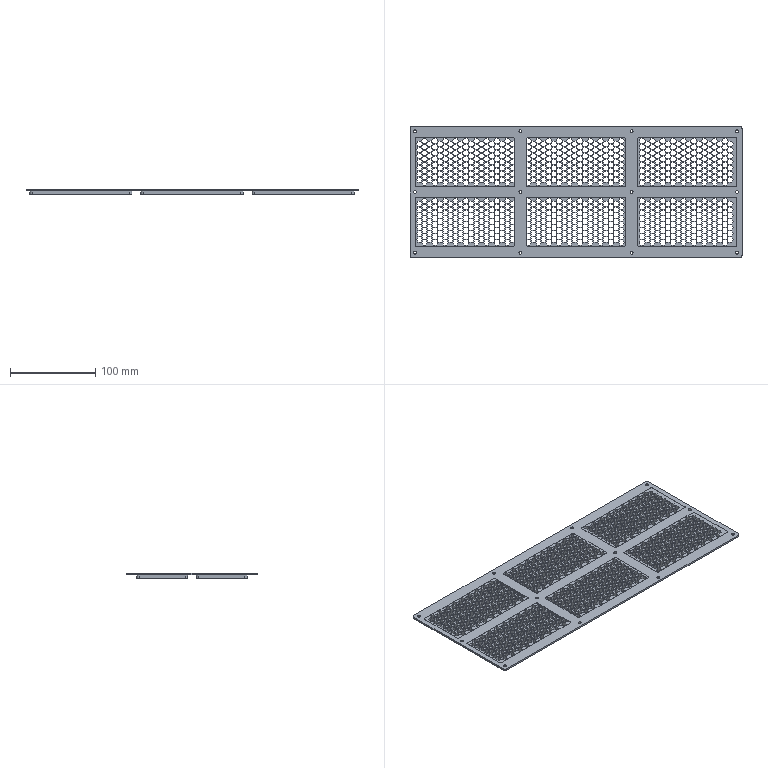NC program | NX | posted with a generic post
Lines 172768 to 172913 of 172913:
(PLANAR_MILL_5 , TOOL : D4_CHAMFER)
N345498 T04 M6
N345500 G54
N345502 G17 G0 G90 X131. Y-66.75 S4500 M3
N345504 G43 Z20. H4
N345506 Z1.
N345508 G94 G1 Z-1. F1000.
N345510 G3 X130. Y-65.75 R1.
N345512 G1 X73.
N345514 G2 X69.25 Y-62. R3.75
N345516 G1 Y-8.
N345518 G2 X73. Y-4.25 R3.75
N345520 G1 X187.
N345522 G2 X190.75 Y-8. R3.75
N345524 G1 Y-62.
N345526 G2 X187. Y-65.75 R3.75
N345528 G1 X130.
N345530 G3 X129. Y-66.75 R1.
N345532 G1 Z1.
N345534 G0 Z20.
N345536 Y66.75
N345538 Z1.
N345540 G1 Z-1.
N345542 G3 X130. Y65.75 R1.
N345544 G1 X187.
N345546 G2 X190.75 Y62. R3.75
N345548 G1 Y8.
N345550 G2 X187. Y4.25 R3.75
N345552 G1 X73.
N345554 G2 X69.25 Y8. R3.75
N345556 G1 Y62.
N345558 G2 X73. Y65.75 R3.75
N345560 G1 X130.
N345562 G3 X131. Y66.75 R1.
N345564 G1 Z1.
N345566 G0 Z20.
N345568 X-1.
N345570 Z1.
N345572 G1 Z-1.
N345574 G3 X0. Y65.75 R1.
N345576 G1 X57.
N345578 G2 X60.75 Y62. R3.75
N345580 G1 Y8.
N345582 G2 X57. Y4.25 R3.75
N345584 G1 X-57.
N345586 G2 X-60.75 Y8. R3.75
N345588 G1 Y62.
N345590 G2 X-57. Y65.75 R3.75
N345592 G1 X0.
N345594 G3 X1. Y66.75 R1.
N345596 G1 Z1.
N345598 G0 Z20.
N345600 Y-66.75
N345602 Z1.
N345604 G1 Z-1.
N345606 G3 X0. Y-65.75 R1.
N345608 G1 X-57.
N345610 G2 X-60.75 Y-62. R3.75
N345612 G1 Y-8.
N345614 G2 X-57. Y-4.25 R3.75
N345616 G1 X57.
N345618 G2 X60.75 Y-8. R3.75
N345620 G1 Y-62.
N345622 G2 X57. Y-65.75 R3.75
N345624 G1 X0.
N345626 G3 X-1. Y-66.75 R1.
N345628 G1 Z1.
N345630 G0 Z20.
N345632 X-129.
N345634 Z1.
N345636 G1 Z-1.
N345638 G3 X-130. Y-65.75 R1.
N345640 G1 X-187.
N345642 G2 X-190.75 Y-62. R3.75
N345644 G1 Y-8.
N345646 G2 X-187. Y-4.25 R3.75
N345648 G1 X-73.
N345650 G2 X-69.25 Y-8. R3.75
N345652 G1 Y-62.
N345654 G2 X-73. Y-65.75 R3.75
N345656 G1 X-130.
N345658 G3 X-131. Y-66.75 R1.
N345660 G1 Z1.
N345662 G0 Z20.
N345664 Y66.75
N345666 Z1.
N345668 G1 Z-1.
N345670 G3 X-130. Y65.75 R1.
N345672 G1 X-73.
N345674 G2 X-69.25 Y62. R3.75
N345676 G1 Y8.
N345678 G2 X-73. Y4.25 R3.75
N345680 G1 X-187.
N345682 G2 X-190.75 Y8. R3.75
N345684 G1 Y62.
N345686 G2 X-187. Y65.75 R3.75
N345688 G1 X-130.
N345690 G3 X-129. Y66.75 R1.
N345692 G1 Z1.
N345694 G0 Z20.
(PLANAR_MILL_5_COPY , TOOL : D4_CHAMFER)
N345696 X-1. Y78.75
N345698 Z-3.5
N345700 G1 Z-5.5
N345702 G3 X0. Y77.75 R1.
N345704 G1 X191.5
N345706 G2 X195.25 Y74. R3.75
N345708 G1 Y-74.
N345710 G2 X191.5 Y-77.75 R3.75
N345712 G1 X-191.5
N345714 G2 X-195.25 Y-74. R3.75
N345716 G1 Y74.
N345718 G2 X-191.5 Y77.75 R3.75
N345720 G1 X0.
N345722 G3 X1. Y78.75 R1.
N345724 G1 Z-3.5
N345726 G0 Z20.
N345728 M5
(PLANAR_MILL_6 , TOOL : D6_FINISH)
N345730 T02 M6
N345732 G54
N345734 G17 G0 G90 X-2. Y81.95 S4500 M3
N345736 G43 Z20. H2
N345738 Z-4.5
N345740 G94 G1 Z-6.5 F1000.
N345742 G3 X0. Y79.95 R2.
N345744 G1 X191.5
N345746 G2 X197.45 Y74. R5.95
N345748 G1 Y-74.
N345750 G2 X191.5 Y-79.95 R5.95
N345752 G1 X-191.5
N345754 G2 X-197.45 Y-74. R5.95
N345756 G1 Y74.
N345758 G2 X-191.5 Y79.95 R5.95
N345760 G1 X0.
N345762 G3 X2. Y81.95 R2.
N345764 G1 Z-4.5
N345766 G0 Z20.
N345768 M5
N345770 M2